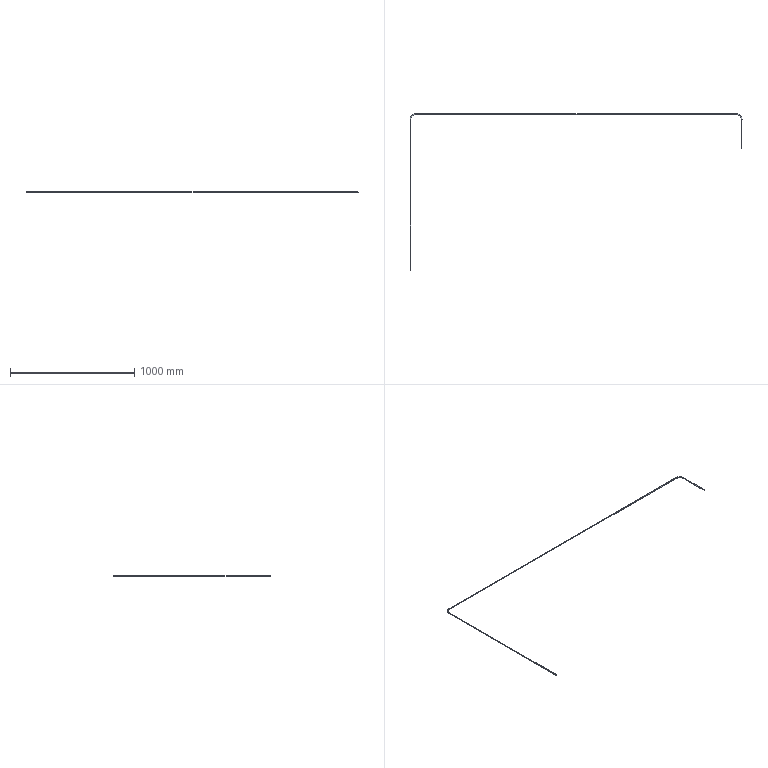Part | SolidWorks | features Sweep 1 | 1 solid | 12 faces | box 2669 x 1258 x 6.5 mm | volume 138073 mm3 | cylinder 6 | torus 4 | plane 2 | commonest cylinder face diameters 6.5 x6
STEP:
#1=CARTESIAN_POINT('',(2620.,1255.,-3.25));
#2=VERTEX_POINT('',#1);
#3=CARTESIAN_POINT('',(2620.,1258.25,0.));
#4=VERTEX_POINT('',#3);
#5=CARTESIAN_POINT('',(2620.,1255.,0.));
#6=DIRECTION('',(1.,0.,0.));
#7=DIRECTION('',(0.,0.,1.));
#8=AXIS2_PLACEMENT_3D('',#5,#6,#7);
#9=CIRCLE('',#8,3.25);
#10=EDGE_CURVE('',#2,#4,#9,.T.);
#11=ORIENTED_EDGE('',*,*,#10,.T.);
#12=CARTESIAN_POINT('',(2665.25,1213.,0.));
#13=VERTEX_POINT('',#12);
#14=CARTESIAN_POINT('',(2620.,1213.,0.));
#15=DIRECTION('',(0.,0.,-1.));
#16=DIRECTION('',(-1.,0.,0.));
#17=AXIS2_PLACEMENT_3D('',#14,#15,#16);
#18=CIRCLE('',#17,45.25);
#19=EDGE_CURVE('',#4,#13,#18,.T.);
#20=ORIENTED_EDGE('',*,*,#19,.T.);
#21=CARTESIAN_POINT('',(2662.,1213.,-3.25));
#22=VERTEX_POINT('',#21);
#23=CARTESIAN_POINT('',(2662.,1213.,0.));
#24=DIRECTION('',(0.,-1.,0.));
#25=DIRECTION('',(0.,0.,1.));
#26=AXIS2_PLACEMENT_3D('',#23,#24,#25);
#27=CIRCLE('',#26,3.25);
#28=EDGE_CURVE('',#22,#13,#27,.T.);
#29=ORIENTED_EDGE('',*,*,#28,.F.);
#30=CARTESIAN_POINT('',(2658.75,1213.,0.));
#31=VERTEX_POINT('',#30);
#32=CARTESIAN_POINT('',(2662.,1213.,0.));
#33=DIRECTION('',(0.,-1.,0.));
#34=DIRECTION('',(0.,0.,1.));
#35=AXIS2_PLACEMENT_3D('',#32,#33,#34);
#36=CIRCLE('',#35,3.25);
#37=EDGE_CURVE('',#31,#22,#36,.T.);
#38=ORIENTED_EDGE('',*,*,#37,.F.);
#39=CARTESIAN_POINT('',(2620.,1251.75,0.));
#40=VERTEX_POINT('',#39);
#41=CARTESIAN_POINT('',(2620.,1213.,0.));
#42=DIRECTION('',(0.,0.,-1.));
#43=DIRECTION('',(-1.,0.,0.));
#44=AXIS2_PLACEMENT_3D('',#41,#42,#43);
#45=CIRCLE('',#44,38.75);
#46=EDGE_CURVE('',#40,#31,#45,.T.);
#47=ORIENTED_EDGE('',*,*,#46,.F.);
#48=CARTESIAN_POINT('',(2620.,1255.,0.));
#49=DIRECTION('',(1.,0.,0.));
#50=DIRECTION('',(0.,0.,1.));
#51=AXIS2_PLACEMENT_3D('',#48,#49,#50);
#52=CIRCLE('',#51,3.25);
#53=EDGE_CURVE('',#40,#2,#52,.T.);
#54=ORIENTED_EDGE('',*,*,#53,.T.);
#55=EDGE_LOOP('',(#11,#20,#29,#38,#47,#54));
#56=FACE_OUTER_BOUND('',#55,.T.);
#57=CARTESIAN_POINT('',(2620.,1213.,0.));
#58=DIRECTION('',(0.,0.,-1.));
#59=DIRECTION('',(-1.,0.,0.));
#60=AXIS2_PLACEMENT_3D('',#57,#58,#59);
#61=TOROIDAL_SURFACE('',#60,42.,3.25);
#62=ADVANCED_FACE('',(#56),#61,.T.);
#63=CARTESIAN_POINT('',(0.,1213.,-3.25));
#64=VERTEX_POINT('',#63);
#65=CARTESIAN_POINT('',(-3.25,1213.,0.));
#66=VERTEX_POINT('',#65);
#67=CARTESIAN_POINT('',(0.,1213.,0.));
#68=DIRECTION('',(0.,1.,0.));
#69=DIRECTION('',(0.,0.,1.));
#70=AXIS2_PLACEMENT_3D('',#67,#68,#69);
#71=CIRCLE('',#70,3.25);
#72=EDGE_CURVE('',#64,#66,#71,.T.);
#73=ORIENTED_EDGE('',*,*,#72,.T.);
#74=CARTESIAN_POINT('',(42.,1258.25,0.));
#75=VERTEX_POINT('',#74);
#76=CARTESIAN_POINT('',(42.,1213.,0.));
#77=DIRECTION('',(0.,0.,-1.));
#78=DIRECTION('',(-1.,0.,0.));
#79=AXIS2_PLACEMENT_3D('',#76,#77,#78);
#80=CIRCLE('',#79,45.25);
#81=EDGE_CURVE('',#66,#75,#80,.T.);
#82=ORIENTED_EDGE('',*,*,#81,.T.);
#83=CARTESIAN_POINT('',(42.,1255.,-3.25));
#84=VERTEX_POINT('',#83);
#85=CARTESIAN_POINT('',(42.,1255.,0.));
#86=DIRECTION('',(1.,0.,0.));
#87=DIRECTION('',(0.,0.,1.));
#88=AXIS2_PLACEMENT_3D('',#85,#86,#87);
#89=CIRCLE('',#88,3.25);
#90=EDGE_CURVE('',#84,#75,#89,.T.);
#91=ORIENTED_EDGE('',*,*,#90,.F.);
#92=CARTESIAN_POINT('',(42.,1251.75,0.));
#93=VERTEX_POINT('',#92);
#94=CARTESIAN_POINT('',(42.,1255.,0.));
#95=DIRECTION('',(1.,0.,0.));
#96=DIRECTION('',(0.,0.,1.));
#97=AXIS2_PLACEMENT_3D('',#94,#95,#96);
#98=CIRCLE('',#97,3.25);
#99=EDGE_CURVE('',#93,#84,#98,.T.);
#100=ORIENTED_EDGE('',*,*,#99,.F.);
#101=CARTESIAN_POINT('',(3.25,1213.,0.));
#102=VERTEX_POINT('',#101);
#103=CARTESIAN_POINT('',(42.,1213.,0.));
#104=DIRECTION('',(0.,0.,-1.));
#105=DIRECTION('',(-1.,0.,0.));
#106=AXIS2_PLACEMENT_3D('',#103,#104,#105);
#107=CIRCLE('',#106,38.75);
#108=EDGE_CURVE('',#102,#93,#107,.T.);
#109=ORIENTED_EDGE('',*,*,#108,.F.);
#110=CARTESIAN_POINT('',(0.,1213.,0.));
#111=DIRECTION('',(0.,1.,0.));
#112=DIRECTION('',(0.,0.,1.));
#113=AXIS2_PLACEMENT_3D('',#110,#111,#112);
#114=CIRCLE('',#113,3.25);
#115=EDGE_CURVE('',#102,#64,#114,.T.);
#116=ORIENTED_EDGE('',*,*,#115,.T.);
#117=EDGE_LOOP('',(#73,#82,#91,#100,#109,#116));
#118=FACE_OUTER_BOUND('',#117,.T.);
#119=CARTESIAN_POINT('',(42.,1213.,0.));
#120=DIRECTION('',(0.,0.,-1.));
#121=DIRECTION('',(-1.,0.,0.));
#122=AXIS2_PLACEMENT_3D('',#119,#120,#121);
#123=TOROIDAL_SURFACE('',#122,42.,3.25);
#124=ADVANCED_FACE('',(#118),#123,.T.);
#125=ORIENTED_EDGE('',*,*,#28,.T.);
#126=CARTESIAN_POINT('',(2662.,1213.,3.25));
#127=VERTEX_POINT('',#126);
#128=CARTESIAN_POINT('',(2662.,1213.,0.));
#129=DIRECTION('',(0.,-1.,0.));
#130=DIRECTION('',(0.,0.,1.));
#131=AXIS2_PLACEMENT_3D('',#128,#129,#130);
#132=CIRCLE('',#131,3.25);
#133=EDGE_CURVE('',#13,#127,#132,.T.);
#134=ORIENTED_EDGE('',*,*,#133,.T.);
#135=CARTESIAN_POINT('',(2662.,975.,3.25));
#136=VERTEX_POINT('',#135);
#137=CARTESIAN_POINT('',(2662.,1213.,3.25));
#138=DIRECTION('',(0.,-1.,0.));
#139=VECTOR('',#138,1000.);
#140=LINE('',#137,#139);
#141=EDGE_CURVE('',#127,#136,#140,.T.);
#142=ORIENTED_EDGE('',*,*,#141,.T.);
#143=CARTESIAN_POINT('',(2662.,975.,-3.25));
#144=VERTEX_POINT('',#143);
#145=CARTESIAN_POINT('',(2662.,975.,0.));
#146=DIRECTION('',(0.,-1.,0.));
#147=DIRECTION('',(0.,0.,1.));
#148=AXIS2_PLACEMENT_3D('',#145,#146,#147);
#149=CIRCLE('',#148,3.25);
#150=EDGE_CURVE('',#144,#136,#149,.T.);
#151=ORIENTED_EDGE('',*,*,#150,.F.);
#152=CARTESIAN_POINT('',(2662.,1213.,-3.25));
#153=DIRECTION('',(0.,-1.,0.));
#154=VECTOR('',#153,1000.);
#155=LINE('',#152,#154);
#156=EDGE_CURVE('',#22,#144,#155,.T.);
#157=ORIENTED_EDGE('',*,*,#156,.F.);
#158=EDGE_LOOP('',(#125,#134,#142,#151,#157));
#159=FACE_OUTER_BOUND('',#158,.T.);
#160=CARTESIAN_POINT('',(2662.,1213.,0.));
#161=DIRECTION('',(0.,-1.,0.));
#162=DIRECTION('',(0.,0.,-1.));
#163=AXIS2_PLACEMENT_3D('',#160,#161,#162);
#164=CYLINDRICAL_SURFACE('',#163,3.25);
#165=ADVANCED_FACE('',(#159),#164,.T.);
#166=ORIENTED_EDGE('',*,*,#90,.T.);
#167=CARTESIAN_POINT('',(42.,1255.,3.25));
#168=VERTEX_POINT('',#167);
#169=CARTESIAN_POINT('',(42.,1255.,0.));
#170=DIRECTION('',(1.,0.,0.));
#171=DIRECTION('',(0.,0.,1.));
#172=AXIS2_PLACEMENT_3D('',#169,#170,#171);
#173=CIRCLE('',#172,3.25);
#174=EDGE_CURVE('',#75,#168,#173,.T.);
#175=ORIENTED_EDGE('',*,*,#174,.T.);
#176=CARTESIAN_POINT('',(2620.,1255.,3.25));
#177=VERTEX_POINT('',#176);
#178=CARTESIAN_POINT('',(42.,1255.,3.25));
#179=DIRECTION('',(1.,0.,0.));
#180=VECTOR('',#179,1000.);
#181=LINE('',#178,#180);
#182=EDGE_CURVE('',#168,#177,#181,.T.);
#183=ORIENTED_EDGE('',*,*,#182,.T.);
#184=CARTESIAN_POINT('',(2620.,1255.,0.));
#185=DIRECTION('',(1.,0.,0.));
#186=DIRECTION('',(0.,0.,1.));
#187=AXIS2_PLACEMENT_3D('',#184,#185,#186);
#188=CIRCLE('',#187,3.25);
#189=EDGE_CURVE('',#4,#177,#188,.T.);
#190=ORIENTED_EDGE('',*,*,#189,.F.);
#191=ORIENTED_EDGE('',*,*,#10,.F.);
#192=CARTESIAN_POINT('',(42.,1255.,-3.25));
#193=DIRECTION('',(1.,0.,0.));
#194=VECTOR('',#193,1000.);
#195=LINE('',#192,#194);
#196=EDGE_CURVE('',#84,#2,#195,.T.);
#197=ORIENTED_EDGE('',*,*,#196,.F.);
#198=EDGE_LOOP('',(#166,#175,#183,#190,#191,#197));
#199=FACE_OUTER_BOUND('',#198,.T.);
#200=CARTESIAN_POINT('',(42.,1255.,0.));
#201=DIRECTION('',(1.,0.,0.));
#202=DIRECTION('',(0.,0.,-1.));
#203=AXIS2_PLACEMENT_3D('',#200,#201,#202);
#204=CYLINDRICAL_SURFACE('',#203,3.25);
#205=ADVANCED_FACE('',(#199),#204,.T.);
#206=CARTESIAN_POINT('',(0.,0.,3.25));
#207=VERTEX_POINT('',#206);
#208=CARTESIAN_POINT('',(0.,0.,-3.25));
#209=VERTEX_POINT('',#208);
#210=CARTESIAN_POINT('',(0.,0.,0.));
#211=DIRECTION('',(0.,1.,0.));
#212=DIRECTION('',(0.,0.,1.));
#213=AXIS2_PLACEMENT_3D('',#210,#211,#212);
#214=CIRCLE('',#213,3.25);
#215=EDGE_CURVE('',#207,#209,#214,.T.);
#216=ORIENTED_EDGE('',*,*,#215,.T.);
#217=CARTESIAN_POINT('',(0.,0.,-3.25));
#218=DIRECTION('',(0.,1.,0.));
#219=VECTOR('',#218,1000.);
#220=LINE('',#217,#219);
#221=EDGE_CURVE('',#209,#64,#220,.T.);
#222=ORIENTED_EDGE('',*,*,#221,.T.);
#223=ORIENTED_EDGE('',*,*,#115,.F.);
#224=CARTESIAN_POINT('',(0.,1213.,3.25));
#225=VERTEX_POINT('',#224);
#226=CARTESIAN_POINT('',(0.,1213.,0.));
#227=DIRECTION('',(0.,1.,0.));
#228=DIRECTION('',(0.,0.,1.));
#229=AXIS2_PLACEMENT_3D('',#226,#227,#228);
#230=CIRCLE('',#229,3.25);
#231=EDGE_CURVE('',#225,#102,#230,.T.);
#232=ORIENTED_EDGE('',*,*,#231,.F.);
#233=CARTESIAN_POINT('',(0.,0.,3.25));
#234=DIRECTION('',(0.,1.,0.));
#235=VECTOR('',#234,1000.);
#236=LINE('',#233,#235);
#237=EDGE_CURVE('',#207,#225,#236,.T.);
#238=ORIENTED_EDGE('',*,*,#237,.F.);
#239=EDGE_LOOP('',(#216,#222,#223,#232,#238));
#240=FACE_OUTER_BOUND('',#239,.T.);
#241=CARTESIAN_POINT('',(0.,0.,0.));
#242=DIRECTION('',(0.,1.,0.));
#243=DIRECTION('',(0.,0.,1.));
#244=AXIS2_PLACEMENT_3D('',#241,#242,#243);
#245=CYLINDRICAL_SURFACE('',#244,3.25);
#246=ADVANCED_FACE('',(#240),#245,.T.);
#247=ORIENTED_EDGE('',*,*,#141,.F.);
#248=CARTESIAN_POINT('',(2662.,1213.,0.));
#249=DIRECTION('',(0.,-1.,0.));
#250=DIRECTION('',(0.,0.,1.));
#251=AXIS2_PLACEMENT_3D('',#248,#249,#250);
#252=CIRCLE('',#251,3.25);
#253=EDGE_CURVE('',#127,#31,#252,.T.);
#254=ORIENTED_EDGE('',*,*,#253,.T.);
#255=ORIENTED_EDGE('',*,*,#37,.T.);
#256=ORIENTED_EDGE('',*,*,#156,.T.);
#257=CARTESIAN_POINT('',(2662.,975.,0.));
#258=DIRECTION('',(0.,-1.,0.));
#259=DIRECTION('',(0.,0.,1.));
#260=AXIS2_PLACEMENT_3D('',#257,#258,#259);
#261=CIRCLE('',#260,3.25);
#262=EDGE_CURVE('',#136,#144,#261,.T.);
#263=ORIENTED_EDGE('',*,*,#262,.F.);
#264=EDGE_LOOP('',(#247,#254,#255,#256,#263));
#265=FACE_OUTER_BOUND('',#264,.T.);
#266=CARTESIAN_POINT('',(2662.,1213.,0.));
#267=DIRECTION('',(0.,-1.,0.));
#268=DIRECTION('',(0.,0.,-1.));
#269=AXIS2_PLACEMENT_3D('',#266,#267,#268);
#270=CYLINDRICAL_SURFACE('',#269,3.25);
#271=ADVANCED_FACE('',(#265),#270,.T.);
#272=ORIENTED_EDGE('',*,*,#19,.F.);
#273=ORIENTED_EDGE('',*,*,#189,.T.);
#274=CARTESIAN_POINT('',(2620.,1255.,0.));
#275=DIRECTION('',(1.,0.,0.));
#276=DIRECTION('',(0.,0.,1.));
#277=AXIS2_PLACEMENT_3D('',#274,#275,#276);
#278=CIRCLE('',#277,3.25);
#279=EDGE_CURVE('',#177,#40,#278,.T.);
#280=ORIENTED_EDGE('',*,*,#279,.T.);
#281=ORIENTED_EDGE('',*,*,#46,.T.);
#282=ORIENTED_EDGE('',*,*,#253,.F.);
#283=ORIENTED_EDGE('',*,*,#133,.F.);
#284=EDGE_LOOP('',(#272,#273,#280,#281,#282,#283));
#285=FACE_OUTER_BOUND('',#284,.T.);
#286=CARTESIAN_POINT('',(2620.,1213.,0.));
#287=DIRECTION('',(0.,0.,-1.));
#288=DIRECTION('',(-1.,0.,0.));
#289=AXIS2_PLACEMENT_3D('',#286,#287,#288);
#290=TOROIDAL_SURFACE('',#289,42.,3.25);
#291=ADVANCED_FACE('',(#285),#290,.T.);
#292=ORIENTED_EDGE('',*,*,#182,.F.);
#293=CARTESIAN_POINT('',(42.,1255.,0.));
#294=DIRECTION('',(1.,0.,0.));
#295=DIRECTION('',(0.,0.,1.));
#296=AXIS2_PLACEMENT_3D('',#293,#294,#295);
#297=CIRCLE('',#296,3.25);
#298=EDGE_CURVE('',#168,#93,#297,.T.);
#299=ORIENTED_EDGE('',*,*,#298,.T.);
#300=ORIENTED_EDGE('',*,*,#99,.T.);
#301=ORIENTED_EDGE('',*,*,#196,.T.);
#302=ORIENTED_EDGE('',*,*,#53,.F.);
#303=ORIENTED_EDGE('',*,*,#279,.F.);
#304=EDGE_LOOP('',(#292,#299,#300,#301,#302,#303));
#305=FACE_OUTER_BOUND('',#304,.T.);
#306=CARTESIAN_POINT('',(42.,1255.,0.));
#307=DIRECTION('',(1.,0.,0.));
#308=DIRECTION('',(0.,0.,-1.));
#309=AXIS2_PLACEMENT_3D('',#306,#307,#308);
#310=CYLINDRICAL_SURFACE('',#309,3.25);
#311=ADVANCED_FACE('',(#305),#310,.T.);
#312=ORIENTED_EDGE('',*,*,#81,.F.);
#313=CARTESIAN_POINT('',(0.,1213.,0.));
#314=DIRECTION('',(0.,1.,0.));
#315=DIRECTION('',(0.,0.,1.));
#316=AXIS2_PLACEMENT_3D('',#313,#314,#315);
#317=CIRCLE('',#316,3.25);
#318=EDGE_CURVE('',#66,#225,#317,.T.);
#319=ORIENTED_EDGE('',*,*,#318,.T.);
#320=ORIENTED_EDGE('',*,*,#231,.T.);
#321=ORIENTED_EDGE('',*,*,#108,.T.);
#322=ORIENTED_EDGE('',*,*,#298,.F.);
#323=ORIENTED_EDGE('',*,*,#174,.F.);
#324=EDGE_LOOP('',(#312,#319,#320,#321,#322,#323));
#325=FACE_OUTER_BOUND('',#324,.T.);
#326=CARTESIAN_POINT('',(42.,1213.,0.));
#327=DIRECTION('',(0.,0.,-1.));
#328=DIRECTION('',(-1.,0.,0.));
#329=AXIS2_PLACEMENT_3D('',#326,#327,#328);
#330=TOROIDAL_SURFACE('',#329,42.,3.25);
#331=ADVANCED_FACE('',(#325),#330,.T.);
#332=ORIENTED_EDGE('',*,*,#221,.F.);
#333=CARTESIAN_POINT('',(0.,0.,0.));
#334=DIRECTION('',(0.,1.,0.));
#335=DIRECTION('',(0.,0.,1.));
#336=AXIS2_PLACEMENT_3D('',#333,#334,#335);
#337=CIRCLE('',#336,3.25);
#338=EDGE_CURVE('',#209,#207,#337,.T.);
#339=ORIENTED_EDGE('',*,*,#338,.T.);
#340=ORIENTED_EDGE('',*,*,#237,.T.);
#341=ORIENTED_EDGE('',*,*,#318,.F.);
#342=ORIENTED_EDGE('',*,*,#72,.F.);
#343=EDGE_LOOP('',(#332,#339,#340,#341,#342));
#344=FACE_OUTER_BOUND('',#343,.T.);
#345=CARTESIAN_POINT('',(0.,0.,0.));
#346=DIRECTION('',(0.,1.,0.));
#347=DIRECTION('',(0.,0.,1.));
#348=AXIS2_PLACEMENT_3D('',#345,#346,#347);
#349=CYLINDRICAL_SURFACE('',#348,3.25);
#350=ADVANCED_FACE('',(#344),#349,.T.);
#351=ORIENTED_EDGE('',*,*,#150,.T.);
#352=ORIENTED_EDGE('',*,*,#262,.T.);
#353=EDGE_LOOP('',(#351,#352));
#354=FACE_OUTER_BOUND('',#353,.T.);
#355=CARTESIAN_POINT('',(2662.,975.,0.));
#356=DIRECTION('',(0.,-1.,0.));
#357=DIRECTION('',(0.,0.,1.));
#358=AXIS2_PLACEMENT_3D('',#355,#356,#357);
#359=PLANE('',#358);
#360=ADVANCED_FACE('',(#354),#359,.T.);
#361=ORIENTED_EDGE('',*,*,#215,.F.);
#362=ORIENTED_EDGE('',*,*,#338,.F.);
#363=EDGE_LOOP('',(#361,#362));
#364=FACE_OUTER_BOUND('',#363,.T.);
#365=CARTESIAN_POINT('',(0.,0.,0.));
#366=DIRECTION('',(0.,1.,0.));
#367=DIRECTION('',(0.,0.,1.));
#368=AXIS2_PLACEMENT_3D('',#365,#366,#367);
#369=PLANE('',#368);
#370=ADVANCED_FACE('',(#364),#369,.F.);
#371=CLOSED_SHELL('',(#62,#124,#165,#205,#246,#271,#291,#311,#331,#350,#360,#370));
#372=MANIFOLD_SOLID_BREP('',#371);
#373=CARTESIAN_POINT('',(0.,0.,0.));
#374=DIRECTION('',(0.,0.,1.));
#375=DIRECTION('',(1.,0.,0.));
#376=AXIS2_PLACEMENT_3D('',#373,#374,#375);
#377=(LENGTH_UNIT()NAMED_UNIT(*)SI_UNIT(.MILLI.,.METRE.));
#378=UNCERTAINTY_MEASURE_WITH_UNIT(LENGTH_MEASURE(0.00001),#377,'','');
#379=(NAMED_UNIT(*)PLANE_ANGLE_UNIT()SI_UNIT($,.RADIAN.));
#380=(NAMED_UNIT(*)SI_UNIT($,.STERADIAN.)SOLID_ANGLE_UNIT());
#381=(GEOMETRIC_REPRESENTATION_CONTEXT(3)GLOBAL_UNCERTAINTY_ASSIGNED_CONTEXT((#378))GLOBAL_UNIT_ASSIGNED_CONTEXT((#377,#379,#380))REPRESENTATION_CONTEXT('',''));
#382=ADVANCED_BREP_SHAPE_REPRESENTATION('',(#372,#376),#381);